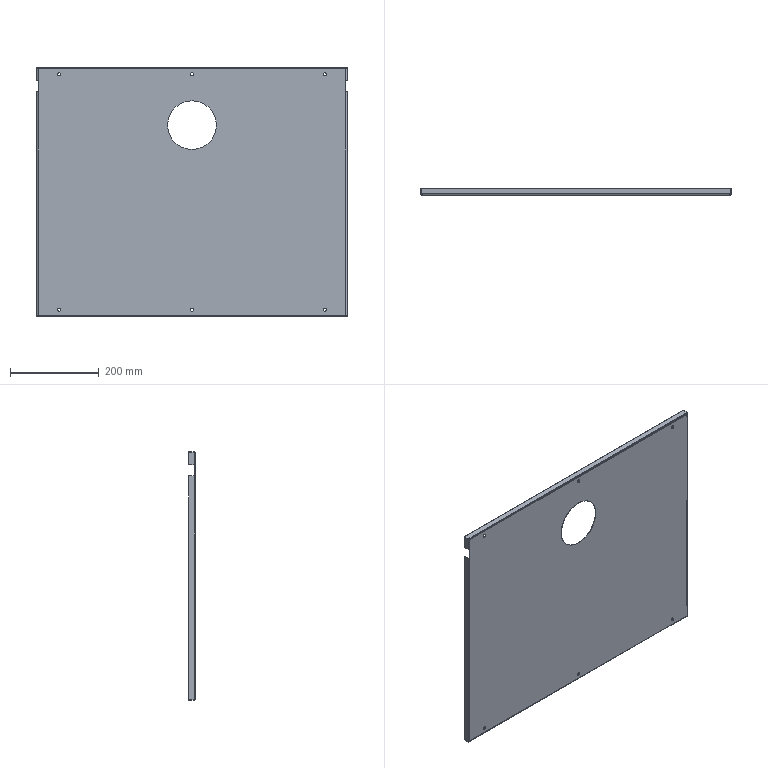Part | STEP file | 1 solid | 84 faces | box 700 x 15 x 562 mm | volume 498385 mm3 | plane 58 | cylinder 26 | commonest cylinder face diameters 7 x12 3 x6 5.4 x6 110 x2